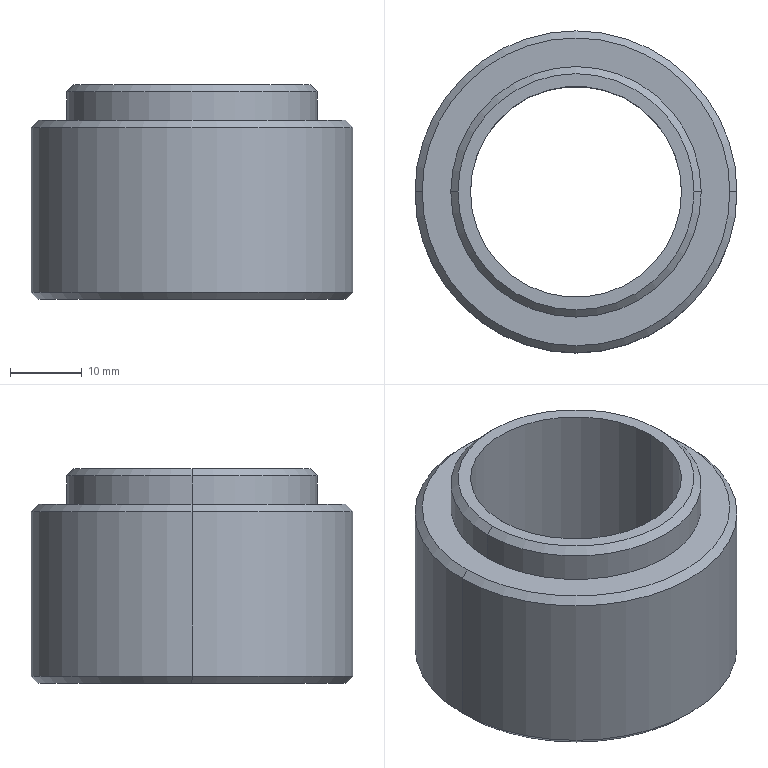Part | SolidWorks | features Chamfer 1, Extrusion 1, ICE 1 | 1 solid | 15 faces | box 45 x 45 x 30 mm | volume 23873 mm3 | cone 6 | cylinder 6 | plane 3 | commonest cylinder face diameters 29.5 x2 35 x2 45 x2
STEP:
#1=CARTESIAN_POINT('',(21.5,0.,25.));
#2=VERTEX_POINT('',#1);
#3=CARTESIAN_POINT('',(-21.5,0.,25.));
#4=VERTEX_POINT('',#3);
#5=CARTESIAN_POINT('',(0.,0.,25.));
#6=DIRECTION('',(0.,0.,1.));
#7=DIRECTION('',(1.,0.,0.));
#8=AXIS2_PLACEMENT_3D('',#5,#6,#7);
#9=CIRCLE('',#8,21.5);
#10=EDGE_CURVE('',#2,#4,#9,.T.);
#11=ORIENTED_EDGE('',*,*,#10,.F.);
#12=CARTESIAN_POINT('',(22.5,0.,24.));
#13=VERTEX_POINT('',#12);
#14=CARTESIAN_POINT('',(21.5,0.,25.));
#15=DIRECTION('',(0.7071,0.,-0.7071));
#16=VECTOR('',#15,1000.);
#17=LINE('',#14,#16);
#18=EDGE_CURVE('',#2,#13,#17,.T.);
#19=ORIENTED_EDGE('',*,*,#18,.T.);
#20=CARTESIAN_POINT('',(-22.5,0.,24.));
#21=VERTEX_POINT('',#20);
#22=CARTESIAN_POINT('',(0.,0.,24.));
#23=DIRECTION('',(0.,0.,-1.));
#24=DIRECTION('',(1.,0.,0.));
#25=AXIS2_PLACEMENT_3D('',#22,#23,#24);
#26=CIRCLE('',#25,22.5);
#27=EDGE_CURVE('',#21,#13,#26,.T.);
#28=ORIENTED_EDGE('',*,*,#27,.F.);
#29=CARTESIAN_POINT('',(-21.5,0.,25.));
#30=DIRECTION('',(-0.7071,0.,-0.7071));
#31=VECTOR('',#30,1000.);
#32=LINE('',#29,#31);
#33=EDGE_CURVE('',#4,#21,#32,.T.);
#34=ORIENTED_EDGE('',*,*,#33,.F.);
#35=EDGE_LOOP('',(#11,#19,#28,#34));
#36=FACE_OUTER_BOUND('',#35,.T.);
#37=CARTESIAN_POINT('',(0.,0.,25.));
#38=DIRECTION('',(0.,0.,-1.));
#39=DIRECTION('',(-1.,0.,0.));
#40=AXIS2_PLACEMENT_3D('',#37,#38,#39);
#41=CONICAL_SURFACE('',#40,21.5,0.7854);
#42=ADVANCED_FACE('',(#36),#41,.T.);
#43=CARTESIAN_POINT('',(-21.5,0.,0.));
#44=VERTEX_POINT('',#43);
#45=CARTESIAN_POINT('',(21.5,0.,0.));
#46=VERTEX_POINT('',#45);
#47=CARTESIAN_POINT('',(0.,0.,0.));
#48=DIRECTION('',(0.,0.,-1.));
#49=DIRECTION('',(1.,0.,0.));
#50=AXIS2_PLACEMENT_3D('',#47,#48,#49);
#51=CIRCLE('',#50,21.5);
#52=EDGE_CURVE('',#44,#46,#51,.T.);
#53=ORIENTED_EDGE('',*,*,#52,.F.);
#54=CARTESIAN_POINT('',(-22.5,0.,1.));
#55=VERTEX_POINT('',#54);
#56=CARTESIAN_POINT('',(-22.5,0.,1.));
#57=DIRECTION('',(-0.7071,0.,0.7071));
#58=VECTOR('',#57,1000.);
#59=LINE('',#56,#58);
#60=EDGE_CURVE('',#44,#55,#59,.T.);
#61=ORIENTED_EDGE('',*,*,#60,.T.);
#62=CARTESIAN_POINT('',(22.5,0.,1.));
#63=VERTEX_POINT('',#62);
#64=CARTESIAN_POINT('',(0.,0.,1.));
#65=DIRECTION('',(0.,0.,1.));
#66=DIRECTION('',(1.,0.,0.));
#67=AXIS2_PLACEMENT_3D('',#64,#65,#66);
#68=CIRCLE('',#67,22.5);
#69=EDGE_CURVE('',#63,#55,#68,.T.);
#70=ORIENTED_EDGE('',*,*,#69,.F.);
#71=CARTESIAN_POINT('',(22.5,0.,1.));
#72=DIRECTION('',(0.7071,0.,0.7071));
#73=VECTOR('',#72,1000.);
#74=LINE('',#71,#73);
#75=EDGE_CURVE('',#46,#63,#74,.T.);
#76=ORIENTED_EDGE('',*,*,#75,.F.);
#77=EDGE_LOOP('',(#53,#61,#70,#76));
#78=FACE_OUTER_BOUND('',#77,.T.);
#79=CARTESIAN_POINT('',(0.,0.,1.));
#80=DIRECTION('',(0.,0.,1.));
#81=DIRECTION('',(1.,0.,0.));
#82=AXIS2_PLACEMENT_3D('',#79,#80,#81);
#83=CONICAL_SURFACE('',#82,22.5,0.7854);
#84=ADVANCED_FACE('',(#78),#83,.T.);
#85=CARTESIAN_POINT('',(16.5,0.,30.));
#86=VERTEX_POINT('',#85);
#87=CARTESIAN_POINT('',(-16.5,0.,30.));
#88=VERTEX_POINT('',#87);
#89=CARTESIAN_POINT('',(0.,0.,30.));
#90=DIRECTION('',(0.,0.,1.));
#91=DIRECTION('',(1.,0.,0.));
#92=AXIS2_PLACEMENT_3D('',#89,#90,#91);
#93=CIRCLE('',#92,16.5);
#94=EDGE_CURVE('',#86,#88,#93,.T.);
#95=ORIENTED_EDGE('',*,*,#94,.F.);
#96=CARTESIAN_POINT('',(17.5,0.,29.));
#97=VERTEX_POINT('',#96);
#98=CARTESIAN_POINT('',(16.5,0.,30.));
#99=DIRECTION('',(0.7071,0.,-0.7071));
#100=VECTOR('',#99,1000.);
#101=LINE('',#98,#100);
#102=EDGE_CURVE('',#86,#97,#101,.T.);
#103=ORIENTED_EDGE('',*,*,#102,.T.);
#104=CARTESIAN_POINT('',(-17.5,0.,29.));
#105=VERTEX_POINT('',#104);
#106=CARTESIAN_POINT('',(0.,0.,29.));
#107=DIRECTION('',(0.,0.,-1.));
#108=DIRECTION('',(1.,0.,0.));
#109=AXIS2_PLACEMENT_3D('',#106,#107,#108);
#110=CIRCLE('',#109,17.5);
#111=EDGE_CURVE('',#105,#97,#110,.T.);
#112=ORIENTED_EDGE('',*,*,#111,.F.);
#113=CARTESIAN_POINT('',(-16.5,0.,30.));
#114=DIRECTION('',(-0.7071,0.,-0.7071));
#115=VECTOR('',#114,1000.);
#116=LINE('',#113,#115);
#117=EDGE_CURVE('',#88,#105,#116,.T.);
#118=ORIENTED_EDGE('',*,*,#117,.F.);
#119=EDGE_LOOP('',(#95,#103,#112,#118));
#120=FACE_OUTER_BOUND('',#119,.T.);
#121=CARTESIAN_POINT('',(0.,0.,30.));
#122=DIRECTION('',(0.,0.,-1.));
#123=DIRECTION('',(-1.,0.,0.));
#124=AXIS2_PLACEMENT_3D('',#121,#122,#123);
#125=CONICAL_SURFACE('',#124,16.5,0.7854);
#126=ADVANCED_FACE('',(#120),#125,.T.);
#127=ORIENTED_EDGE('',*,*,#111,.T.);
#128=CARTESIAN_POINT('',(17.5,0.,25.));
#129=VERTEX_POINT('',#128);
#130=CARTESIAN_POINT('',(17.5,0.,30.));
#131=DIRECTION('',(0.,0.,-1.));
#132=VECTOR('',#131,1000.);
#133=LINE('',#130,#132);
#134=EDGE_CURVE('',#97,#129,#133,.T.);
#135=ORIENTED_EDGE('',*,*,#134,.T.);
#136=CARTESIAN_POINT('',(-17.5,0.,25.));
#137=VERTEX_POINT('',#136);
#138=CARTESIAN_POINT('',(0.,0.,25.));
#139=DIRECTION('',(0.,0.,1.));
#140=DIRECTION('',(1.,0.,0.));
#141=AXIS2_PLACEMENT_3D('',#138,#139,#140);
#142=CIRCLE('',#141,17.5);
#143=EDGE_CURVE('',#129,#137,#142,.T.);
#144=ORIENTED_EDGE('',*,*,#143,.T.);
#145=CARTESIAN_POINT('',(-17.5,0.,30.));
#146=DIRECTION('',(0.,0.,-1.));
#147=VECTOR('',#146,1000.);
#148=LINE('',#145,#147);
#149=EDGE_CURVE('',#105,#137,#148,.T.);
#150=ORIENTED_EDGE('',*,*,#149,.F.);
#151=EDGE_LOOP('',(#127,#135,#144,#150));
#152=FACE_OUTER_BOUND('',#151,.T.);
#153=CARTESIAN_POINT('',(0.,0.,30.));
#154=DIRECTION('',(0.,0.,-1.));
#155=DIRECTION('',(-1.,0.,0.));
#156=AXIS2_PLACEMENT_3D('',#153,#154,#155);
#157=CYLINDRICAL_SURFACE('',#156,17.5);
#158=ADVANCED_FACE('',(#152),#157,.T.);
#159=CARTESIAN_POINT('',(-14.75,0.,30.));
#160=VERTEX_POINT('',#159);
#161=CARTESIAN_POINT('',(14.75,0.,30.));
#162=VERTEX_POINT('',#161);
#163=CARTESIAN_POINT('',(0.,0.,30.));
#164=DIRECTION('',(0.,0.,1.));
#165=DIRECTION('',(1.,0.,0.));
#166=AXIS2_PLACEMENT_3D('',#163,#164,#165);
#167=CIRCLE('',#166,14.75);
#168=EDGE_CURVE('',#160,#162,#167,.T.);
#169=ORIENTED_EDGE('',*,*,#168,.T.);
#170=CARTESIAN_POINT('',(14.75,0.,0.));
#171=VERTEX_POINT('',#170);
#172=CARTESIAN_POINT('',(14.75,0.,25.));
#173=DIRECTION('',(0.,0.,-1.));
#174=VECTOR('',#173,1000.);
#175=LINE('',#172,#174);
#176=EDGE_CURVE('',#162,#171,#175,.T.);
#177=ORIENTED_EDGE('',*,*,#176,.T.);
#178=CARTESIAN_POINT('',(-14.75,0.,0.));
#179=VERTEX_POINT('',#178);
#180=CARTESIAN_POINT('',(0.,0.,0.));
#181=DIRECTION('',(0.,0.,1.));
#182=DIRECTION('',(1.,0.,0.));
#183=AXIS2_PLACEMENT_3D('',#180,#181,#182);
#184=CIRCLE('',#183,14.75);
#185=EDGE_CURVE('',#179,#171,#184,.T.);
#186=ORIENTED_EDGE('',*,*,#185,.F.);
#187=CARTESIAN_POINT('',(-14.75,0.,25.));
#188=DIRECTION('',(0.,0.,-1.));
#189=VECTOR('',#188,1000.);
#190=LINE('',#187,#189);
#191=EDGE_CURVE('',#160,#179,#190,.T.);
#192=ORIENTED_EDGE('',*,*,#191,.F.);
#193=EDGE_LOOP('',(#169,#177,#186,#192));
#194=FACE_OUTER_BOUND('',#193,.T.);
#195=CARTESIAN_POINT('',(0.,0.,25.));
#196=DIRECTION('',(0.,0.,-1.));
#197=DIRECTION('',(-1.,0.,0.));
#198=AXIS2_PLACEMENT_3D('',#195,#196,#197);
#199=CYLINDRICAL_SURFACE('',#198,14.75);
#200=ADVANCED_FACE('',(#194),#199,.F.);
#201=ORIENTED_EDGE('',*,*,#27,.T.);
#202=CARTESIAN_POINT('',(22.5,0.,25.));
#203=DIRECTION('',(0.,0.,-1.));
#204=VECTOR('',#203,1000.);
#205=LINE('',#202,#204);
#206=EDGE_CURVE('',#13,#63,#205,.T.);
#207=ORIENTED_EDGE('',*,*,#206,.T.);
#208=ORIENTED_EDGE('',*,*,#69,.T.);
#209=CARTESIAN_POINT('',(-22.5,0.,25.));
#210=DIRECTION('',(0.,0.,-1.));
#211=VECTOR('',#210,1000.);
#212=LINE('',#209,#211);
#213=EDGE_CURVE('',#21,#55,#212,.T.);
#214=ORIENTED_EDGE('',*,*,#213,.F.);
#215=EDGE_LOOP('',(#201,#207,#208,#214));
#216=FACE_OUTER_BOUND('',#215,.T.);
#217=CARTESIAN_POINT('',(0.,0.,25.));
#218=DIRECTION('',(0.,0.,-1.));
#219=DIRECTION('',(-1.,0.,0.));
#220=AXIS2_PLACEMENT_3D('',#217,#218,#219);
#221=CYLINDRICAL_SURFACE('',#220,22.5);
#222=ADVANCED_FACE('',(#216),#221,.T.);
#223=CARTESIAN_POINT('',(0.,0.,25.));
#224=DIRECTION('',(0.,0.,1.));
#225=DIRECTION('',(1.,0.,0.));
#226=AXIS2_PLACEMENT_3D('',#223,#224,#225);
#227=CIRCLE('',#226,21.5);
#228=EDGE_CURVE('',#4,#2,#227,.T.);
#229=ORIENTED_EDGE('',*,*,#228,.T.);
#230=ORIENTED_EDGE('',*,*,#10,.T.);
#231=EDGE_LOOP('',(#229,#230));
#232=FACE_OUTER_BOUND('',#231,.T.);
#233=CARTESIAN_POINT('',(0.,0.,25.));
#234=DIRECTION('',(0.,0.,1.));
#235=DIRECTION('',(1.,0.,0.));
#236=AXIS2_PLACEMENT_3D('',#233,#234,#235);
#237=CIRCLE('',#236,17.5);
#238=EDGE_CURVE('',#137,#129,#237,.T.);
#239=ORIENTED_EDGE('',*,*,#238,.F.);
#240=ORIENTED_EDGE('',*,*,#143,.F.);
#241=EDGE_LOOP('',(#239,#240));
#242=FACE_BOUND('',#241,.T.);
#243=CARTESIAN_POINT('',(0.,0.,25.));
#244=DIRECTION('',(0.,0.,1.));
#245=DIRECTION('',(1.,0.,0.));
#246=AXIS2_PLACEMENT_3D('',#243,#244,#245);
#247=PLANE('',#246);
#248=ADVANCED_FACE('',(#232,#242),#247,.T.);
#249=CARTESIAN_POINT('',(0.,0.,0.));
#250=DIRECTION('',(0.,0.,-1.));
#251=DIRECTION('',(1.,0.,0.));
#252=AXIS2_PLACEMENT_3D('',#249,#250,#251);
#253=CIRCLE('',#252,21.5);
#254=EDGE_CURVE('',#46,#44,#253,.T.);
#255=ORIENTED_EDGE('',*,*,#254,.T.);
#256=ORIENTED_EDGE('',*,*,#52,.T.);
#257=EDGE_LOOP('',(#255,#256));
#258=FACE_OUTER_BOUND('',#257,.T.);
#259=ORIENTED_EDGE('',*,*,#185,.T.);
#260=CARTESIAN_POINT('',(0.,0.,0.));
#261=DIRECTION('',(0.,0.,1.));
#262=DIRECTION('',(1.,0.,0.));
#263=AXIS2_PLACEMENT_3D('',#260,#261,#262);
#264=CIRCLE('',#263,14.75);
#265=EDGE_CURVE('',#171,#179,#264,.T.);
#266=ORIENTED_EDGE('',*,*,#265,.T.);
#267=EDGE_LOOP('',(#259,#266));
#268=FACE_BOUND('',#267,.T.);
#269=CARTESIAN_POINT('',(0.,0.,0.));
#270=DIRECTION('',(0.,0.,1.));
#271=DIRECTION('',(1.,0.,0.));
#272=AXIS2_PLACEMENT_3D('',#269,#270,#271);
#273=PLANE('',#272);
#274=ADVANCED_FACE('',(#258,#268),#273,.F.);
#275=ORIENTED_EDGE('',*,*,#206,.F.);
#276=CARTESIAN_POINT('',(0.,0.,24.));
#277=DIRECTION('',(0.,0.,-1.));
#278=DIRECTION('',(1.,0.,0.));
#279=AXIS2_PLACEMENT_3D('',#276,#277,#278);
#280=CIRCLE('',#279,22.5);
#281=EDGE_CURVE('',#13,#21,#280,.T.);
#282=ORIENTED_EDGE('',*,*,#281,.T.);
#283=ORIENTED_EDGE('',*,*,#213,.T.);
#284=CARTESIAN_POINT('',(0.,0.,1.));
#285=DIRECTION('',(0.,0.,1.));
#286=DIRECTION('',(1.,0.,0.));
#287=AXIS2_PLACEMENT_3D('',#284,#285,#286);
#288=CIRCLE('',#287,22.5);
#289=EDGE_CURVE('',#55,#63,#288,.T.);
#290=ORIENTED_EDGE('',*,*,#289,.T.);
#291=EDGE_LOOP('',(#275,#282,#283,#290));
#292=FACE_OUTER_BOUND('',#291,.T.);
#293=CARTESIAN_POINT('',(0.,0.,25.));
#294=DIRECTION('',(0.,0.,-1.));
#295=DIRECTION('',(-1.,0.,0.));
#296=AXIS2_PLACEMENT_3D('',#293,#294,#295);
#297=CYLINDRICAL_SURFACE('',#296,22.5);
#298=ADVANCED_FACE('',(#292),#297,.T.);
#299=ORIENTED_EDGE('',*,*,#176,.F.);
#300=CARTESIAN_POINT('',(0.,0.,30.));
#301=DIRECTION('',(0.,0.,1.));
#302=DIRECTION('',(1.,0.,0.));
#303=AXIS2_PLACEMENT_3D('',#300,#301,#302);
#304=CIRCLE('',#303,14.75);
#305=EDGE_CURVE('',#162,#160,#304,.T.);
#306=ORIENTED_EDGE('',*,*,#305,.T.);
#307=ORIENTED_EDGE('',*,*,#191,.T.);
#308=ORIENTED_EDGE('',*,*,#265,.F.);
#309=EDGE_LOOP('',(#299,#306,#307,#308));
#310=FACE_OUTER_BOUND('',#309,.T.);
#311=CARTESIAN_POINT('',(0.,0.,25.));
#312=DIRECTION('',(0.,0.,-1.));
#313=DIRECTION('',(-1.,0.,0.));
#314=AXIS2_PLACEMENT_3D('',#311,#312,#313);
#315=CYLINDRICAL_SURFACE('',#314,14.75);
#316=ADVANCED_FACE('',(#310),#315,.F.);
#317=CARTESIAN_POINT('',(0.,0.,30.));
#318=DIRECTION('',(0.,0.,1.));
#319=DIRECTION('',(1.,0.,0.));
#320=AXIS2_PLACEMENT_3D('',#317,#318,#319);
#321=CIRCLE('',#320,16.5);
#322=EDGE_CURVE('',#88,#86,#321,.T.);
#323=ORIENTED_EDGE('',*,*,#322,.T.);
#324=ORIENTED_EDGE('',*,*,#94,.T.);
#325=EDGE_LOOP('',(#323,#324));
#326=FACE_OUTER_BOUND('',#325,.T.);
#327=ORIENTED_EDGE('',*,*,#168,.F.);
#328=ORIENTED_EDGE('',*,*,#305,.F.);
#329=EDGE_LOOP('',(#327,#328));
#330=FACE_BOUND('',#329,.T.);
#331=CARTESIAN_POINT('',(0.,0.,30.));
#332=DIRECTION('',(0.,0.,1.));
#333=DIRECTION('',(1.,0.,0.));
#334=AXIS2_PLACEMENT_3D('',#331,#332,#333);
#335=PLANE('',#334);
#336=ADVANCED_FACE('',(#326,#330),#335,.T.);
#337=ORIENTED_EDGE('',*,*,#134,.F.);
#338=CARTESIAN_POINT('',(0.,0.,29.));
#339=DIRECTION('',(0.,0.,-1.));
#340=DIRECTION('',(1.,0.,0.));
#341=AXIS2_PLACEMENT_3D('',#338,#339,#340);
#342=CIRCLE('',#341,17.5);
#343=EDGE_CURVE('',#97,#105,#342,.T.);
#344=ORIENTED_EDGE('',*,*,#343,.T.);
#345=ORIENTED_EDGE('',*,*,#149,.T.);
#346=ORIENTED_EDGE('',*,*,#238,.T.);
#347=EDGE_LOOP('',(#337,#344,#345,#346));
#348=FACE_OUTER_BOUND('',#347,.T.);
#349=CARTESIAN_POINT('',(0.,0.,30.));
#350=DIRECTION('',(0.,0.,-1.));
#351=DIRECTION('',(-1.,0.,0.));
#352=AXIS2_PLACEMENT_3D('',#349,#350,#351);
#353=CYLINDRICAL_SURFACE('',#352,17.5);
#354=ADVANCED_FACE('',(#348),#353,.T.);
#355=ORIENTED_EDGE('',*,*,#102,.F.);
#356=ORIENTED_EDGE('',*,*,#322,.F.);
#357=ORIENTED_EDGE('',*,*,#117,.T.);
#358=ORIENTED_EDGE('',*,*,#343,.F.);
#359=EDGE_LOOP('',(#355,#356,#357,#358));
#360=FACE_OUTER_BOUND('',#359,.T.);
#361=CARTESIAN_POINT('',(0.,0.,30.));
#362=DIRECTION('',(0.,0.,-1.));
#363=DIRECTION('',(-1.,0.,0.));
#364=AXIS2_PLACEMENT_3D('',#361,#362,#363);
#365=CONICAL_SURFACE('',#364,16.5,0.7854);
#366=ADVANCED_FACE('',(#360),#365,.T.);
#367=ORIENTED_EDGE('',*,*,#60,.F.);
#368=ORIENTED_EDGE('',*,*,#254,.F.);
#369=ORIENTED_EDGE('',*,*,#75,.T.);
#370=ORIENTED_EDGE('',*,*,#289,.F.);
#371=EDGE_LOOP('',(#367,#368,#369,#370));
#372=FACE_OUTER_BOUND('',#371,.T.);
#373=CARTESIAN_POINT('',(0.,0.,1.));
#374=DIRECTION('',(0.,0.,1.));
#375=DIRECTION('',(1.,0.,0.));
#376=AXIS2_PLACEMENT_3D('',#373,#374,#375);
#377=CONICAL_SURFACE('',#376,22.5,0.7854);
#378=ADVANCED_FACE('',(#372),#377,.T.);
#379=ORIENTED_EDGE('',*,*,#18,.F.);
#380=ORIENTED_EDGE('',*,*,#228,.F.);
#381=ORIENTED_EDGE('',*,*,#33,.T.);
#382=ORIENTED_EDGE('',*,*,#281,.F.);
#383=EDGE_LOOP('',(#379,#380,#381,#382));
#384=FACE_OUTER_BOUND('',#383,.T.);
#385=CARTESIAN_POINT('',(0.,0.,25.));
#386=DIRECTION('',(0.,0.,-1.));
#387=DIRECTION('',(-1.,0.,0.));
#388=AXIS2_PLACEMENT_3D('',#385,#386,#387);
#389=CONICAL_SURFACE('',#388,21.5,0.7854);
#390=ADVANCED_FACE('',(#384),#389,.T.);
#391=CLOSED_SHELL('',(#42,#84,#126,#158,#200,#222,#248,#274,#298,#316,#336,#354,#366,#378,#390));
#392=MANIFOLD_SOLID_BREP('',#391);
#393=CARTESIAN_POINT('',(0.,0.,0.));
#394=DIRECTION('',(0.,0.,1.));
#395=DIRECTION('',(1.,0.,0.));
#396=AXIS2_PLACEMENT_3D('',#393,#394,#395);
#397=(LENGTH_UNIT()NAMED_UNIT(*)SI_UNIT(.MILLI.,.METRE.));
#398=UNCERTAINTY_MEASURE_WITH_UNIT(LENGTH_MEASURE(0.00001),#397,'','');
#399=(NAMED_UNIT(*)PLANE_ANGLE_UNIT()SI_UNIT($,.RADIAN.));
#400=(NAMED_UNIT(*)SI_UNIT($,.STERADIAN.)SOLID_ANGLE_UNIT());
#401=(GEOMETRIC_REPRESENTATION_CONTEXT(3)GLOBAL_UNCERTAINTY_ASSIGNED_CONTEXT((#398))GLOBAL_UNIT_ASSIGNED_CONTEXT((#397,#399,#400))REPRESENTATION_CONTEXT('',''));
#402=ADVANCED_BREP_SHAPE_REPRESENTATION('',(#392,#396),#401);